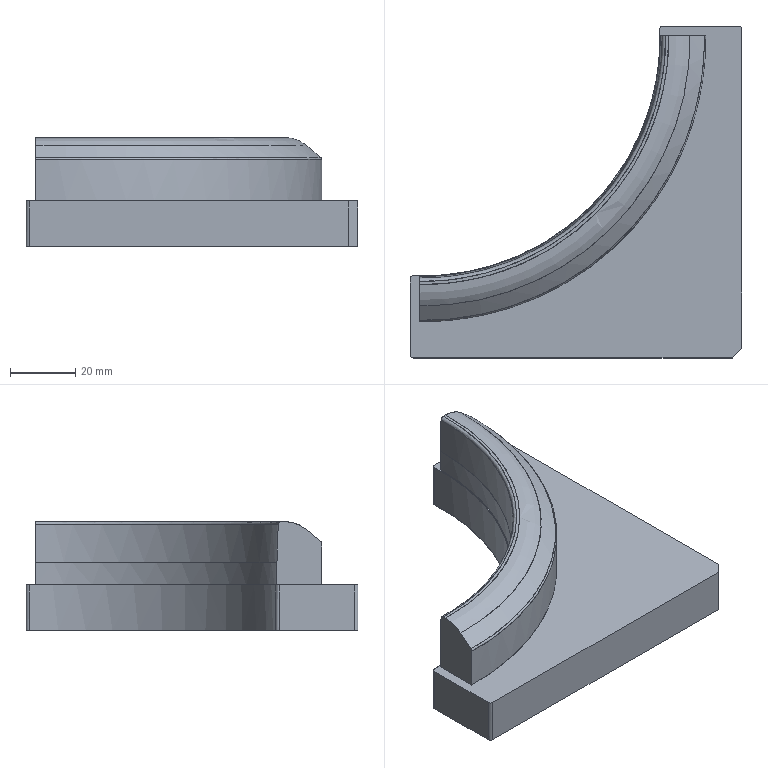NC program | PowerMill | posted with a generic post | part box 102 x 102 x 33.478 mm
Lines 205716 to 205885 of 205885:
N205813 M6
N205814 S15000 M03
N205815 G00 G90 X0.0 Y0.0
N205816 G43 Z10.298 H13
N205817
N205818 G05 P10000 R8
N205819 X-21.4567 Y-47.0628
N205820 Z-19.63
N205821 G01 Z-19.73 F600.0
N205822 X-21.4036 Y-46.7435 F1000.0
N205823 X-21.307 Y-46.4639
N205824 X-21.1668 Y-46.2239
N205825 X-20.9831 Y-46.0234
N205826 X-20.7602 Y-45.8654
N205827 X-20.5026 Y-45.7525
N205828 X-20.2101 Y-45.6848
N205829 X-19.8829 Y-45.6623
N205830 X-19.5777 Y-45.6839
N205831 X-19.2997 Y-45.7489
N205832 X-19.0488 Y-45.8571
N205833 X-18.8251 Y-46.0087
N205834 X-18.6284 Y-46.2107
N205835 X-18.4879 Y-46.4445
N205836 X-18.4036 Y-46.7101
N205837 X-18.3755 Y-47.0075
N205838 X-18.3976 Y-47.2229
N205839 X-18.4639 Y-47.4416
N205840 X-18.5745 Y-47.6636
N205841 X-18.7127 Y-47.8294
N205842 X-18.9947 Y-48.1059
N205843 X-19.1183 Y-48.189
N205844 X-19.3174 Y-48.2811
N205845 X-19.9622 Y-48.5302
N205846 X-20.3031 Y-48.7122
N205847 X-20.6145 Y-48.9282
N205848 X-20.8965 Y-49.1784
N205849 X-21.1637 Y-49.4862
N205850 X-21.3646 Y-49.8123
N205851 X-21.4991 Y-50.157
N205852 X-21.5673 Y-50.52
N205853 X-18.3718
N205854 G00 Z-16.5904
N205855 G01 X-14.8101 Y-46.3109 F10000.0
N205856 G00 Z-19.63
N205857 G01 Z-19.73 F600.0
N205858 X-13.8998 Y-45.6844 F1000.0
N205859 Y-50.52
N205860 G00 Z-16.5904
N205861 G01 X-9.0149 Y-48.8135 F10000.0
N205862 G00 Z-19.63
N205863 G01 Z-19.73 F600.0
N205864 X-10.8688 F1000.0
N205865 G00 Z-16.5904
N205866 G01 X-2.7001 Y-50.52 F10000.0
N205867 G00 Z-19.63
N205868 G01 Z-19.73 F600.0
N205869 X-4.9926 Y-45.6659 F1000.0
N205870 X-7.2077 Y-50.52
N205871 G00 Z-16.5904
N205872 G01 X-3.6122 Y-48.5887 F10000.0
N205873 G00 Z-19.63
N205874 G01 Z-19.73 F600.0
N205875 X-6.312 F1000.0
N205876 G00 Z-16.5904
N205877 G01 X0.939 Y-48.8135 F10000.0
N205878 G00 Z-19.63
N205879 G01 Z-19.73 F600.0
N205880 X-0.9149 F1000.0
N205881 G00 Z-16.5904
N205882 G01 X4.3496 Y-46.3109 F10000.0
N205883 G00 Z-19.63
N205884 G01 Z-19.73 F600.0
N205885 X5.2599 Y-45.6844 F1000.0
N205886 Y-50.52
N205887 G00 Z-16.5904
N205888 G01 X10.1447 Y-48.8135 F10000.0
N205889 G00 Z-19.63
N205890 G01 Z-19.73 F600.0
N205891 X8.2908 F1000.0
N205892 G00 Z-16.5904
N205893 G01 X12.2516 Y-48.6529 F10000.0
N205894 G00 Z-19.63
N205895 G01 Z-19.73 F600.0
N205896 X12.2321 Y-48.1354 F1000.0
N205897 X12.2516 Y-47.6163
N205898 X12.31 Y-47.1583
N205899 X12.4074 Y-46.7614
N205900 X12.5437 Y-46.4256
N205901 X12.719 Y-46.1508
N205902 X12.9332 Y-45.937
N205903 X13.1864 Y-45.7844
N205904 X13.4785 Y-45.6928
N205905 X13.8096 Y-45.6623
N205906 X14.1407 Y-45.6928
N205907 X14.4328 Y-45.7844
N205908 X14.686 Y-45.937
N205909 X14.9002 Y-46.1508
N205910 X15.0755 Y-46.4256
N205911 X15.2118 Y-46.7614
N205912 X15.3092 Y-47.1583
N205913 X15.3676 Y-47.6163
N205914 X15.3871 Y-48.1354
N205915 X15.3676 Y-48.6434
N205916 X15.3093 Y-49.0936
N205917 X15.212 Y-49.4862
N205918 X15.0759 Y-49.8209
N205919 X14.9008 Y-50.098
N205920 X14.6868 Y-50.3173
N205921 X14.4354 Y-50.475
N205922 X14.143 Y-50.5696
N205923 X13.8096 Y-50.6011
N205924 X13.4785 Y-50.5706
N205925 X13.1864 Y-50.4793
N205926 X12.9332 Y-50.3271
N205927 X12.719 Y-50.114
N205928 X12.5437 Y-49.8401
N205929 X12.4074 Y-49.5052
N205930 X12.31 Y-49.1095
N205931 X12.2516 Y-48.6529
N205932 G00 Z-16.5904
N205933 G01 X18.219 Y-50.2767 F10000.0
N205934 G00 Z-19.63
N205935 G01 Z-19.73 F600.0
N205936 Y-49.6074 F1000.0
N205937 G00 Z-16.5904
N205938 G01 X21.0988 Y-47.0628 F10000.0
N205939 G00 Z-19.63
N205940 G01 Z-19.73 F600.0
N205941 X21.1519 Y-46.7435 F1000.0
N205942 X21.2485 Y-46.4639
N205943 X21.3887 Y-46.2239
N205944 X21.5724 Y-46.0234
N205945 X21.7953 Y-45.8654
N205946 X22.0529 Y-45.7525
N205947 X22.3454 Y-45.6848
N205948 X22.6726 Y-45.6623
N205949 X22.9778 Y-45.6839
N205950 X23.2558 Y-45.7489
N205951 X23.5067 Y-45.8571
N205952 X23.7304 Y-46.0087
N205953 X23.9271 Y-46.2107
N205954 X24.0676 Y-46.4445
N205955 X24.1519 Y-46.7101
N205956 X24.18 Y-47.0075
N205957 X24.1579 Y-47.2229
N205958 X24.0916 Y-47.4416
N205959 X23.981 Y-47.6636
N205960 X23.8428 Y-47.8294
N205961 X23.5608 Y-48.1059
N205962 X23.4372 Y-48.189
N205963 X23.2381 Y-48.2811
N205964 X22.5933 Y-48.5302
N205965 X22.2524 Y-48.7122
N205966 X21.941 Y-48.9282
N205967 X21.659 Y-49.1784
N205968 X21.3918 Y-49.4862
N205969 X21.1909 Y-49.8123
N205970 X21.0564 Y-50.157
N205971 X20.9882 Y-50.52
N205972 X24.1837
N205973 G00 Z10.298
N205974 G05 P0
N205975 (---------------)
N205976 ( END TOOLPATH : 粗公刻字01-刻字-TEXT_D4 )
N205977 (---------------)
N205978
N205979 M05
N205980 G53 Z0.0
N205981 M30
%